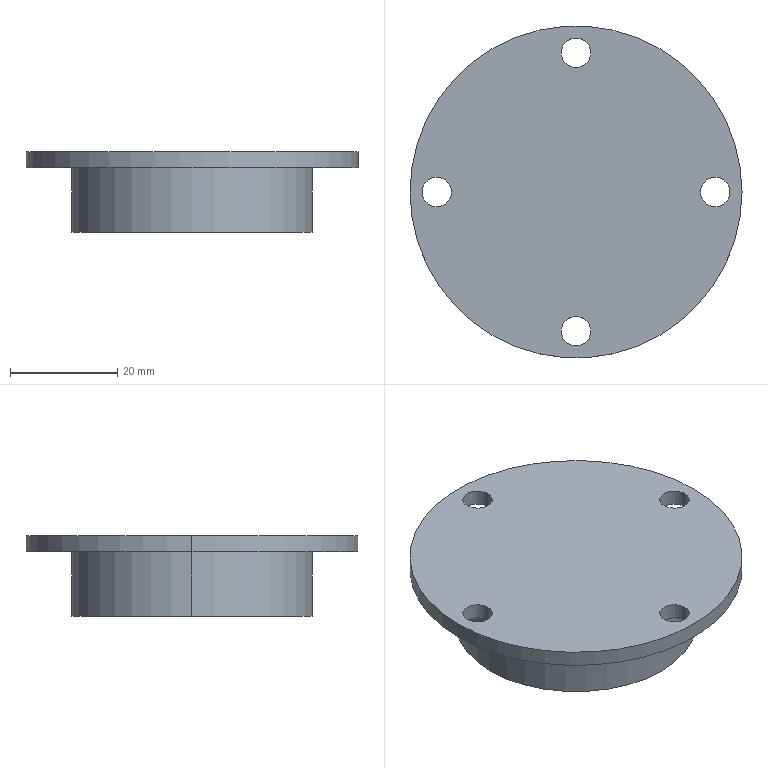Part | SolidWorks | features ICE 2, Cut 1, Extrusion 1 | 1 solid | 18 faces | box 62 x 62 x 15 mm | volume 19198 mm3 | cylinder 14 | plane 4 | commonest cylinder face diameters 5.5 x8 35 x2 45 x2 62 x2
STEP:
#1=CARTESIAN_POINT('',(-52.75,26.,-694.19));
#2=VERTEX_POINT('',#1);
#3=CARTESIAN_POINT('',(-47.25,26.,-694.19));
#4=VERTEX_POINT('',#3);
#5=CARTESIAN_POINT('',(-50.,26.,-694.19));
#6=DIRECTION('',(0.,0.,1.));
#7=DIRECTION('',(1.,0.,0.));
#8=AXIS2_PLACEMENT_3D('',#5,#6,#7);
#9=CIRCLE('',#8,2.75);
#10=EDGE_CURVE('',#2,#4,#9,.T.);
#11=ORIENTED_EDGE('',*,*,#10,.F.);
#12=CARTESIAN_POINT('',(-52.75,26.,-691.19));
#13=VERTEX_POINT('',#12);
#14=CARTESIAN_POINT('',(-52.75,26.,-703.19));
#15=DIRECTION('',(0.,0.,1.));
#16=VECTOR('',#15,1000.);
#17=LINE('',#14,#16);
#18=EDGE_CURVE('',#2,#13,#17,.T.);
#19=ORIENTED_EDGE('',*,*,#18,.T.);
#20=CARTESIAN_POINT('',(-47.25,26.,-691.19));
#21=VERTEX_POINT('',#20);
#22=CARTESIAN_POINT('',(-50.,26.,-691.19));
#23=DIRECTION('',(0.,0.,1.));
#24=DIRECTION('',(1.,0.,0.));
#25=AXIS2_PLACEMENT_3D('',#22,#23,#24);
#26=CIRCLE('',#25,2.75);
#27=EDGE_CURVE('',#13,#21,#26,.T.);
#28=ORIENTED_EDGE('',*,*,#27,.T.);
#29=CARTESIAN_POINT('',(-47.25,26.,-703.19));
#30=DIRECTION('',(0.,0.,1.));
#31=VECTOR('',#30,1000.);
#32=LINE('',#29,#31);
#33=EDGE_CURVE('',#4,#21,#32,.T.);
#34=ORIENTED_EDGE('',*,*,#33,.F.);
#35=EDGE_LOOP('',(#11,#19,#28,#34));
#36=FACE_OUTER_BOUND('',#35,.T.);
#37=CARTESIAN_POINT('',(-50.,26.,-703.19));
#38=DIRECTION('',(0.,0.,1.));
#39=DIRECTION('',(1.,0.,0.));
#40=AXIS2_PLACEMENT_3D('',#37,#38,#39);
#41=CYLINDRICAL_SURFACE('',#40,2.75);
#42=ADVANCED_FACE('',(#36),#41,.F.);
#43=CARTESIAN_POINT('',(-26.75,0.,-694.19));
#44=VERTEX_POINT('',#43);
#45=CARTESIAN_POINT('',(-21.25,0.,-694.19));
#46=VERTEX_POINT('',#45);
#47=CARTESIAN_POINT('',(-24.,0.,-694.19));
#48=DIRECTION('',(0.,0.,1.));
#49=DIRECTION('',(1.,0.,0.));
#50=AXIS2_PLACEMENT_3D('',#47,#48,#49);
#51=CIRCLE('',#50,2.75);
#52=EDGE_CURVE('',#44,#46,#51,.T.);
#53=ORIENTED_EDGE('',*,*,#52,.F.);
#54=CARTESIAN_POINT('',(-26.75,0.,-691.19));
#55=VERTEX_POINT('',#54);
#56=CARTESIAN_POINT('',(-26.75,0.,-703.19));
#57=DIRECTION('',(0.,0.,1.));
#58=VECTOR('',#57,1000.);
#59=LINE('',#56,#58);
#60=EDGE_CURVE('',#44,#55,#59,.T.);
#61=ORIENTED_EDGE('',*,*,#60,.T.);
#62=CARTESIAN_POINT('',(-21.25,0.,-691.19));
#63=VERTEX_POINT('',#62);
#64=CARTESIAN_POINT('',(-24.,0.,-691.19));
#65=DIRECTION('',(0.,0.,1.));
#66=DIRECTION('',(1.,0.,0.));
#67=AXIS2_PLACEMENT_3D('',#64,#65,#66);
#68=CIRCLE('',#67,2.75);
#69=EDGE_CURVE('',#55,#63,#68,.T.);
#70=ORIENTED_EDGE('',*,*,#69,.T.);
#71=CARTESIAN_POINT('',(-21.25,0.,-703.19));
#72=DIRECTION('',(0.,0.,1.));
#73=VECTOR('',#72,1000.);
#74=LINE('',#71,#73);
#75=EDGE_CURVE('',#46,#63,#74,.T.);
#76=ORIENTED_EDGE('',*,*,#75,.F.);
#77=EDGE_LOOP('',(#53,#61,#70,#76));
#78=FACE_OUTER_BOUND('',#77,.T.);
#79=CARTESIAN_POINT('',(-24.,0.,-703.19));
#80=DIRECTION('',(0.,0.,1.));
#81=DIRECTION('',(1.,0.,0.));
#82=AXIS2_PLACEMENT_3D('',#79,#80,#81);
#83=CYLINDRICAL_SURFACE('',#82,2.75);
#84=ADVANCED_FACE('',(#78),#83,.F.);
#85=CARTESIAN_POINT('',(-52.75,-26.,-694.19));
#86=VERTEX_POINT('',#85);
#87=CARTESIAN_POINT('',(-47.25,-26.,-694.19));
#88=VERTEX_POINT('',#87);
#89=CARTESIAN_POINT('',(-50.,-26.,-694.19));
#90=DIRECTION('',(0.,0.,1.));
#91=DIRECTION('',(1.,0.,0.));
#92=AXIS2_PLACEMENT_3D('',#89,#90,#91);
#93=CIRCLE('',#92,2.75);
#94=EDGE_CURVE('',#86,#88,#93,.T.);
#95=ORIENTED_EDGE('',*,*,#94,.F.);
#96=CARTESIAN_POINT('',(-52.75,-26.,-691.19));
#97=VERTEX_POINT('',#96);
#98=CARTESIAN_POINT('',(-52.75,-26.,-703.19));
#99=DIRECTION('',(0.,0.,1.));
#100=VECTOR('',#99,1000.);
#101=LINE('',#98,#100);
#102=EDGE_CURVE('',#86,#97,#101,.T.);
#103=ORIENTED_EDGE('',*,*,#102,.T.);
#104=CARTESIAN_POINT('',(-47.25,-26.,-691.19));
#105=VERTEX_POINT('',#104);
#106=CARTESIAN_POINT('',(-50.,-26.,-691.19));
#107=DIRECTION('',(0.,0.,1.));
#108=DIRECTION('',(1.,0.,0.));
#109=AXIS2_PLACEMENT_3D('',#106,#107,#108);
#110=CIRCLE('',#109,2.75);
#111=EDGE_CURVE('',#97,#105,#110,.T.);
#112=ORIENTED_EDGE('',*,*,#111,.T.);
#113=CARTESIAN_POINT('',(-47.25,-26.,-703.19));
#114=DIRECTION('',(0.,0.,1.));
#115=VECTOR('',#114,1000.);
#116=LINE('',#113,#115);
#117=EDGE_CURVE('',#88,#105,#116,.T.);
#118=ORIENTED_EDGE('',*,*,#117,.F.);
#119=EDGE_LOOP('',(#95,#103,#112,#118));
#120=FACE_OUTER_BOUND('',#119,.T.);
#121=CARTESIAN_POINT('',(-50.,-26.,-703.19));
#122=DIRECTION('',(0.,0.,1.));
#123=DIRECTION('',(1.,0.,0.));
#124=AXIS2_PLACEMENT_3D('',#121,#122,#123);
#125=CYLINDRICAL_SURFACE('',#124,2.75);
#126=ADVANCED_FACE('',(#120),#125,.F.);
#127=CARTESIAN_POINT('',(-78.75,0.,-694.19));
#128=VERTEX_POINT('',#127);
#129=CARTESIAN_POINT('',(-73.25,0.,-694.19));
#130=VERTEX_POINT('',#129);
#131=CARTESIAN_POINT('',(-76.,0.,-694.19));
#132=DIRECTION('',(0.,0.,1.));
#133=DIRECTION('',(1.,0.,0.));
#134=AXIS2_PLACEMENT_3D('',#131,#132,#133);
#135=CIRCLE('',#134,2.75);
#136=EDGE_CURVE('',#128,#130,#135,.T.);
#137=ORIENTED_EDGE('',*,*,#136,.F.);
#138=CARTESIAN_POINT('',(-78.75,0.,-691.19));
#139=VERTEX_POINT('',#138);
#140=CARTESIAN_POINT('',(-78.75,0.,-703.19));
#141=DIRECTION('',(0.,0.,1.));
#142=VECTOR('',#141,1000.);
#143=LINE('',#140,#142);
#144=EDGE_CURVE('',#128,#139,#143,.T.);
#145=ORIENTED_EDGE('',*,*,#144,.T.);
#146=CARTESIAN_POINT('',(-73.25,0.,-691.19));
#147=VERTEX_POINT('',#146);
#148=CARTESIAN_POINT('',(-76.,0.,-691.19));
#149=DIRECTION('',(0.,0.,1.));
#150=DIRECTION('',(1.,0.,0.));
#151=AXIS2_PLACEMENT_3D('',#148,#149,#150);
#152=CIRCLE('',#151,2.75);
#153=EDGE_CURVE('',#139,#147,#152,.T.);
#154=ORIENTED_EDGE('',*,*,#153,.T.);
#155=CARTESIAN_POINT('',(-73.25,0.,-703.19));
#156=DIRECTION('',(0.,0.,1.));
#157=VECTOR('',#156,1000.);
#158=LINE('',#155,#157);
#159=EDGE_CURVE('',#130,#147,#158,.T.);
#160=ORIENTED_EDGE('',*,*,#159,.F.);
#161=EDGE_LOOP('',(#137,#145,#154,#160));
#162=FACE_OUTER_BOUND('',#161,.T.);
#163=CARTESIAN_POINT('',(-76.,0.,-703.19));
#164=DIRECTION('',(0.,0.,1.));
#165=DIRECTION('',(1.,0.,0.));
#166=AXIS2_PLACEMENT_3D('',#163,#164,#165);
#167=CYLINDRICAL_SURFACE('',#166,2.75);
#168=ADVANCED_FACE('',(#162),#167,.F.);
#169=CARTESIAN_POINT('',(-32.5,0.,-697.19));
#170=VERTEX_POINT('',#169);
#171=CARTESIAN_POINT('',(-67.5,0.,-697.19));
#172=VERTEX_POINT('',#171);
#173=CARTESIAN_POINT('',(-50.,0.,-697.19));
#174=DIRECTION('',(0.,0.,-1.));
#175=DIRECTION('',(-1.,0.,0.));
#176=AXIS2_PLACEMENT_3D('',#173,#174,#175);
#177=CIRCLE('',#176,17.5);
#178=EDGE_CURVE('',#170,#172,#177,.T.);
#179=ORIENTED_EDGE('',*,*,#178,.F.);
#180=CARTESIAN_POINT('',(-32.5,0.,-706.19));
#181=VERTEX_POINT('',#180);
#182=CARTESIAN_POINT('',(-32.5,0.,-697.19));
#183=DIRECTION('',(0.,0.,-1.));
#184=VECTOR('',#183,1000.);
#185=LINE('',#182,#184);
#186=EDGE_CURVE('',#170,#181,#185,.T.);
#187=ORIENTED_EDGE('',*,*,#186,.T.);
#188=CARTESIAN_POINT('',(-67.5,0.,-706.19));
#189=VERTEX_POINT('',#188);
#190=CARTESIAN_POINT('',(-50.,0.,-706.19));
#191=DIRECTION('',(0.,0.,-1.));
#192=DIRECTION('',(-1.,0.,0.));
#193=AXIS2_PLACEMENT_3D('',#190,#191,#192);
#194=CIRCLE('',#193,17.5);
#195=EDGE_CURVE('',#181,#189,#194,.T.);
#196=ORIENTED_EDGE('',*,*,#195,.T.);
#197=CARTESIAN_POINT('',(-67.5,0.,-697.19));
#198=DIRECTION('',(0.,0.,-1.));
#199=VECTOR('',#198,1000.);
#200=LINE('',#197,#199);
#201=EDGE_CURVE('',#172,#189,#200,.T.);
#202=ORIENTED_EDGE('',*,*,#201,.F.);
#203=EDGE_LOOP('',(#179,#187,#196,#202));
#204=FACE_OUTER_BOUND('',#203,.T.);
#205=CARTESIAN_POINT('',(-50.,0.,-697.19));
#206=DIRECTION('',(0.,0.,-1.));
#207=DIRECTION('',(-1.,0.,0.));
#208=AXIS2_PLACEMENT_3D('',#205,#206,#207);
#209=CYLINDRICAL_SURFACE('',#208,17.5);
#210=ADVANCED_FACE('',(#204),#209,.F.);
#211=CARTESIAN_POINT('',(-72.5,0.,-706.19));
#212=VERTEX_POINT('',#211);
#213=CARTESIAN_POINT('',(-27.5,0.,-706.19));
#214=VERTEX_POINT('',#213);
#215=CARTESIAN_POINT('',(-50.,0.,-706.19));
#216=DIRECTION('',(0.,0.,-1.));
#217=DIRECTION('',(-1.,0.,0.));
#218=AXIS2_PLACEMENT_3D('',#215,#216,#217);
#219=CIRCLE('',#218,22.5);
#220=EDGE_CURVE('',#212,#214,#219,.T.);
#221=ORIENTED_EDGE('',*,*,#220,.F.);
#222=CARTESIAN_POINT('',(-72.5,0.,-694.19));
#223=VERTEX_POINT('',#222);
#224=CARTESIAN_POINT('',(-72.5,0.,-706.19));
#225=DIRECTION('',(0.,0.,1.));
#226=VECTOR('',#225,1000.);
#227=LINE('',#224,#226);
#228=EDGE_CURVE('',#212,#223,#227,.T.);
#229=ORIENTED_EDGE('',*,*,#228,.T.);
#230=CARTESIAN_POINT('',(-27.5,0.,-694.19));
#231=VERTEX_POINT('',#230);
#232=CARTESIAN_POINT('',(-50.,0.,-694.19));
#233=DIRECTION('',(0.,0.,-1.));
#234=DIRECTION('',(-1.,0.,0.));
#235=AXIS2_PLACEMENT_3D('',#232,#233,#234);
#236=CIRCLE('',#235,22.5);
#237=EDGE_CURVE('',#223,#231,#236,.T.);
#238=ORIENTED_EDGE('',*,*,#237,.T.);
#239=CARTESIAN_POINT('',(-27.5,0.,-706.19));
#240=DIRECTION('',(0.,0.,1.));
#241=VECTOR('',#240,1000.);
#242=LINE('',#239,#241);
#243=EDGE_CURVE('',#214,#231,#242,.T.);
#244=ORIENTED_EDGE('',*,*,#243,.F.);
#245=EDGE_LOOP('',(#221,#229,#238,#244));
#246=FACE_OUTER_BOUND('',#245,.T.);
#247=CARTESIAN_POINT('',(-50.,0.,-706.19));
#248=DIRECTION('',(0.,0.,1.));
#249=DIRECTION('',(1.,0.,0.));
#250=AXIS2_PLACEMENT_3D('',#247,#248,#249);
#251=CYLINDRICAL_SURFACE('',#250,22.5);
#252=ADVANCED_FACE('',(#246),#251,.T.);
#253=CARTESIAN_POINT('',(-19.,0.,-691.19));
#254=VERTEX_POINT('',#253);
#255=CARTESIAN_POINT('',(-81.,0.,-691.19));
#256=VERTEX_POINT('',#255);
#257=CARTESIAN_POINT('',(-50.,0.,-691.19));
#258=DIRECTION('',(0.,0.,1.));
#259=DIRECTION('',(1.,0.,0.));
#260=AXIS2_PLACEMENT_3D('',#257,#258,#259);
#261=CIRCLE('',#260,31.);
#262=EDGE_CURVE('',#254,#256,#261,.T.);
#263=ORIENTED_EDGE('',*,*,#262,.F.);
#264=CARTESIAN_POINT('',(-19.,0.,-694.19));
#265=VERTEX_POINT('',#264);
#266=CARTESIAN_POINT('',(-19.,0.,-691.19));
#267=DIRECTION('',(0.,0.,-1.));
#268=VECTOR('',#267,1000.);
#269=LINE('',#266,#268);
#270=EDGE_CURVE('',#254,#265,#269,.T.);
#271=ORIENTED_EDGE('',*,*,#270,.T.);
#272=CARTESIAN_POINT('',(-81.,0.,-694.19));
#273=VERTEX_POINT('',#272);
#274=CARTESIAN_POINT('',(-50.,0.,-694.19));
#275=DIRECTION('',(0.,0.,1.));
#276=DIRECTION('',(1.,0.,0.));
#277=AXIS2_PLACEMENT_3D('',#274,#275,#276);
#278=CIRCLE('',#277,31.);
#279=EDGE_CURVE('',#265,#273,#278,.T.);
#280=ORIENTED_EDGE('',*,*,#279,.T.);
#281=CARTESIAN_POINT('',(-81.,0.,-691.19));
#282=DIRECTION('',(0.,0.,-1.));
#283=VECTOR('',#282,1000.);
#284=LINE('',#281,#283);
#285=EDGE_CURVE('',#256,#273,#284,.T.);
#286=ORIENTED_EDGE('',*,*,#285,.F.);
#287=EDGE_LOOP('',(#263,#271,#280,#286));
#288=FACE_OUTER_BOUND('',#287,.T.);
#289=CARTESIAN_POINT('',(-50.,0.,-691.19));
#290=DIRECTION('',(0.,0.,-1.));
#291=DIRECTION('',(-1.,0.,0.));
#292=AXIS2_PLACEMENT_3D('',#289,#290,#291);
#293=CYLINDRICAL_SURFACE('',#292,31.);
#294=ADVANCED_FACE('',(#288),#293,.T.);
#295=ORIENTED_EDGE('',*,*,#270,.F.);
#296=CARTESIAN_POINT('',(-50.,0.,-691.19));
#297=DIRECTION('',(0.,0.,1.));
#298=DIRECTION('',(1.,0.,0.));
#299=AXIS2_PLACEMENT_3D('',#296,#297,#298);
#300=CIRCLE('',#299,31.);
#301=EDGE_CURVE('',#256,#254,#300,.T.);
#302=ORIENTED_EDGE('',*,*,#301,.F.);
#303=ORIENTED_EDGE('',*,*,#285,.T.);
#304=CARTESIAN_POINT('',(-50.,0.,-694.19));
#305=DIRECTION('',(0.,0.,1.));
#306=DIRECTION('',(1.,0.,0.));
#307=AXIS2_PLACEMENT_3D('',#304,#305,#306);
#308=CIRCLE('',#307,31.);
#309=EDGE_CURVE('',#273,#265,#308,.T.);
#310=ORIENTED_EDGE('',*,*,#309,.T.);
#311=EDGE_LOOP('',(#295,#302,#303,#310));
#312=FACE_OUTER_BOUND('',#311,.T.);
#313=CARTESIAN_POINT('',(-50.,0.,-691.19));
#314=DIRECTION('',(0.,0.,-1.));
#315=DIRECTION('',(-1.,0.,0.));
#316=AXIS2_PLACEMENT_3D('',#313,#314,#315);
#317=CYLINDRICAL_SURFACE('',#316,31.);
#318=ADVANCED_FACE('',(#312),#317,.T.);
#319=CARTESIAN_POINT('',(-50.,26.,-691.19));
#320=DIRECTION('',(0.,0.,1.));
#321=DIRECTION('',(1.,0.,0.));
#322=AXIS2_PLACEMENT_3D('',#319,#320,#321);
#323=CIRCLE('',#322,2.75);
#324=EDGE_CURVE('',#21,#13,#323,.T.);
#325=ORIENTED_EDGE('',*,*,#324,.F.);
#326=ORIENTED_EDGE('',*,*,#27,.F.);
#327=EDGE_LOOP('',(#325,#326));
#328=FACE_BOUND('',#327,.T.);
#329=CARTESIAN_POINT('',(-24.,0.,-691.19));
#330=DIRECTION('',(0.,0.,1.));
#331=DIRECTION('',(1.,0.,0.));
#332=AXIS2_PLACEMENT_3D('',#329,#330,#331);
#333=CIRCLE('',#332,2.75);
#334=EDGE_CURVE('',#63,#55,#333,.T.);
#335=ORIENTED_EDGE('',*,*,#334,.F.);
#336=ORIENTED_EDGE('',*,*,#69,.F.);
#337=EDGE_LOOP('',(#335,#336));
#338=FACE_BOUND('',#337,.T.);
#339=CARTESIAN_POINT('',(-50.,-26.,-691.19));
#340=DIRECTION('',(0.,0.,1.));
#341=DIRECTION('',(1.,0.,0.));
#342=AXIS2_PLACEMENT_3D('',#339,#340,#341);
#343=CIRCLE('',#342,2.75);
#344=EDGE_CURVE('',#105,#97,#343,.T.);
#345=ORIENTED_EDGE('',*,*,#344,.F.);
#346=ORIENTED_EDGE('',*,*,#111,.F.);
#347=EDGE_LOOP('',(#345,#346));
#348=FACE_BOUND('',#347,.T.);
#349=CARTESIAN_POINT('',(-76.,0.,-691.19));
#350=DIRECTION('',(0.,0.,1.));
#351=DIRECTION('',(1.,0.,0.));
#352=AXIS2_PLACEMENT_3D('',#349,#350,#351);
#353=CIRCLE('',#352,2.75);
#354=EDGE_CURVE('',#147,#139,#353,.T.);
#355=ORIENTED_EDGE('',*,*,#354,.F.);
#356=ORIENTED_EDGE('',*,*,#153,.F.);
#357=EDGE_LOOP('',(#355,#356));
#358=FACE_BOUND('',#357,.T.);
#359=ORIENTED_EDGE('',*,*,#301,.T.);
#360=ORIENTED_EDGE('',*,*,#262,.T.);
#361=EDGE_LOOP('',(#359,#360));
#362=FACE_OUTER_BOUND('',#361,.T.);
#363=CARTESIAN_POINT('',(-50.,0.,-691.19));
#364=DIRECTION('',(0.,0.,1.));
#365=DIRECTION('',(1.,0.,0.));
#366=AXIS2_PLACEMENT_3D('',#363,#364,#365);
#367=PLANE('',#366);
#368=ADVANCED_FACE('',(#328,#338,#348,#358,#362),#367,.T.);
#369=CARTESIAN_POINT('',(-50.,26.,-694.19));
#370=DIRECTION('',(0.,0.,1.));
#371=DIRECTION('',(1.,0.,0.));
#372=AXIS2_PLACEMENT_3D('',#369,#370,#371);
#373=CIRCLE('',#372,2.75);
#374=EDGE_CURVE('',#4,#2,#373,.T.);
#375=ORIENTED_EDGE('',*,*,#374,.T.);
#376=ORIENTED_EDGE('',*,*,#10,.T.);
#377=EDGE_LOOP('',(#375,#376));
#378=FACE_BOUND('',#377,.T.);
#379=CARTESIAN_POINT('',(-24.,0.,-694.19));
#380=DIRECTION('',(0.,0.,1.));
#381=DIRECTION('',(1.,0.,0.));
#382=AXIS2_PLACEMENT_3D('',#379,#380,#381);
#383=CIRCLE('',#382,2.75);
#384=EDGE_CURVE('',#46,#44,#383,.T.);
#385=ORIENTED_EDGE('',*,*,#384,.T.);
#386=ORIENTED_EDGE('',*,*,#52,.T.);
#387=EDGE_LOOP('',(#385,#386));
#388=FACE_BOUND('',#387,.T.);
#389=CARTESIAN_POINT('',(-50.,-26.,-694.19));
#390=DIRECTION('',(0.,0.,1.));
#391=DIRECTION('',(1.,0.,0.));
#392=AXIS2_PLACEMENT_3D('',#389,#390,#391);
#393=CIRCLE('',#392,2.75);
#394=EDGE_CURVE('',#88,#86,#393,.T.);
#395=ORIENTED_EDGE('',*,*,#394,.T.);
#396=ORIENTED_EDGE('',*,*,#94,.T.);
#397=EDGE_LOOP('',(#395,#396));
#398=FACE_BOUND('',#397,.T.);
#399=CARTESIAN_POINT('',(-76.,0.,-694.19));
#400=DIRECTION('',(0.,0.,1.));
#401=DIRECTION('',(1.,0.,0.));
#402=AXIS2_PLACEMENT_3D('',#399,#400,#401);
#403=CIRCLE('',#402,2.75);
#404=EDGE_CURVE('',#130,#128,#403,.T.);
#405=ORIENTED_EDGE('',*,*,#404,.T.);
#406=ORIENTED_EDGE('',*,*,#136,.T.);
#407=EDGE_LOOP('',(#405,#406));
#408=FACE_BOUND('',#407,.T.);
#409=CARTESIAN_POINT('',(-50.,0.,-694.19));
#410=DIRECTION('',(0.,0.,-1.));
#411=DIRECTION('',(-1.,0.,0.));
#412=AXIS2_PLACEMENT_3D('',#409,#410,#411);
#413=CIRCLE('',#412,22.5);
#414=EDGE_CURVE('',#231,#223,#413,.T.);
#415=ORIENTED_EDGE('',*,*,#414,.F.);
#416=ORIENTED_EDGE('',*,*,#237,.F.);
#417=EDGE_LOOP('',(#415,#416));
#418=FACE_BOUND('',#417,.T.);
#419=ORIENTED_EDGE('',*,*,#309,.F.);
#420=ORIENTED_EDGE('',*,*,#279,.F.);
#421=EDGE_LOOP('',(#419,#420));
#422=FACE_OUTER_BOUND('',#421,.T.);
#423=CARTESIAN_POINT('',(-50.,0.,-694.19));
#424=DIRECTION('',(0.,0.,1.));
#425=DIRECTION('',(1.,0.,0.));
#426=AXIS2_PLACEMENT_3D('',#423,#424,#425);
#427=PLANE('',#426);
#428=ADVANCED_FACE('',(#378,#388,#398,#408,#418,#422),#427,.F.);
#429=ORIENTED_EDGE('',*,*,#228,.F.);
#430=CARTESIAN_POINT('',(-50.,0.,-706.19));
#431=DIRECTION('',(0.,0.,-1.));
#432=DIRECTION('',(-1.,0.,0.));
#433=AXIS2_PLACEMENT_3D('',#430,#431,#432);
#434=CIRCLE('',#433,22.5);
#435=EDGE_CURVE('',#214,#212,#434,.T.);
#436=ORIENTED_EDGE('',*,*,#435,.F.);
#437=ORIENTED_EDGE('',*,*,#243,.T.);
#438=ORIENTED_EDGE('',*,*,#414,.T.);
#439=EDGE_LOOP('',(#429,#436,#437,#438));
#440=FACE_OUTER_BOUND('',#439,.T.);
#441=CARTESIAN_POINT('',(-50.,0.,-706.19));
#442=DIRECTION('',(0.,0.,1.));
#443=DIRECTION('',(1.,0.,0.));
#444=AXIS2_PLACEMENT_3D('',#441,#442,#443);
#445=CYLINDRICAL_SURFACE('',#444,22.5);
#446=ADVANCED_FACE('',(#440),#445,.T.);
#447=CARTESIAN_POINT('',(-50.,0.,-706.19));
#448=DIRECTION('',(0.,0.,-1.));
#449=DIRECTION('',(-1.,0.,0.));
#450=AXIS2_PLACEMENT_3D('',#447,#448,#449);
#451=CIRCLE('',#450,17.5);
#452=EDGE_CURVE('',#189,#181,#451,.T.);
#453=ORIENTED_EDGE('',*,*,#452,.F.);
#454=ORIENTED_EDGE('',*,*,#195,.F.);
#455=EDGE_LOOP('',(#453,#454));
#456=FACE_BOUND('',#455,.T.);
#457=ORIENTED_EDGE('',*,*,#435,.T.);
#458=ORIENTED_EDGE('',*,*,#220,.T.);
#459=EDGE_LOOP('',(#457,#458));
#460=FACE_OUTER_BOUND('',#459,.T.);
#461=CARTESIAN_POINT('',(-50.,0.,-706.19));
#462=DIRECTION('',(0.,0.,-1.));
#463=DIRECTION('',(-1.,0.,0.));
#464=AXIS2_PLACEMENT_3D('',#461,#462,#463);
#465=PLANE('',#464);
#466=ADVANCED_FACE('',(#456,#460),#465,.T.);
#467=ORIENTED_EDGE('',*,*,#186,.F.);
#468=CARTESIAN_POINT('',(-50.,0.,-697.19));
#469=DIRECTION('',(0.,0.,-1.));
#470=DIRECTION('',(-1.,0.,0.));
#471=AXIS2_PLACEMENT_3D('',#468,#469,#470);
#472=CIRCLE('',#471,17.5);
#473=EDGE_CURVE('',#172,#170,#472,.T.);
#474=ORIENTED_EDGE('',*,*,#473,.F.);
#475=ORIENTED_EDGE('',*,*,#201,.T.);
#476=ORIENTED_EDGE('',*,*,#452,.T.);
#477=EDGE_LOOP('',(#467,#474,#475,#476));
#478=FACE_OUTER_BOUND('',#477,.T.);
#479=CARTESIAN_POINT('',(-50.,0.,-697.19));
#480=DIRECTION('',(0.,0.,-1.));
#481=DIRECTION('',(-1.,0.,0.));
#482=AXIS2_PLACEMENT_3D('',#479,#480,#481);
#483=CYLINDRICAL_SURFACE('',#482,17.5);
#484=ADVANCED_FACE('',(#478),#483,.F.);
#485=ORIENTED_EDGE('',*,*,#473,.T.);
#486=ORIENTED_EDGE('',*,*,#178,.T.);
#487=EDGE_LOOP('',(#485,#486));
#488=FACE_OUTER_BOUND('',#487,.T.);
#489=CARTESIAN_POINT('',(-50.,0.,-697.19));
#490=DIRECTION('',(0.,0.,-1.));
#491=DIRECTION('',(-1.,0.,0.));
#492=AXIS2_PLACEMENT_3D('',#489,#490,#491);
#493=PLANE('',#492);
#494=ADVANCED_FACE('',(#488),#493,.T.);
#495=ORIENTED_EDGE('',*,*,#144,.F.);
#496=ORIENTED_EDGE('',*,*,#404,.F.);
#497=ORIENTED_EDGE('',*,*,#159,.T.);
#498=ORIENTED_EDGE('',*,*,#354,.T.);
#499=EDGE_LOOP('',(#495,#496,#497,#498));
#500=FACE_OUTER_BOUND('',#499,.T.);
#501=CARTESIAN_POINT('',(-76.,0.,-703.19));
#502=DIRECTION('',(0.,0.,1.));
#503=DIRECTION('',(1.,0.,0.));
#504=AXIS2_PLACEMENT_3D('',#501,#502,#503);
#505=CYLINDRICAL_SURFACE('',#504,2.75);
#506=ADVANCED_FACE('',(#500),#505,.F.);
#507=ORIENTED_EDGE('',*,*,#102,.F.);
#508=ORIENTED_EDGE('',*,*,#394,.F.);
#509=ORIENTED_EDGE('',*,*,#117,.T.);
#510=ORIENTED_EDGE('',*,*,#344,.T.);
#511=EDGE_LOOP('',(#507,#508,#509,#510));
#512=FACE_OUTER_BOUND('',#511,.T.);
#513=CARTESIAN_POINT('',(-50.,-26.,-703.19));
#514=DIRECTION('',(0.,0.,1.));
#515=DIRECTION('',(1.,0.,0.));
#516=AXIS2_PLACEMENT_3D('',#513,#514,#515);
#517=CYLINDRICAL_SURFACE('',#516,2.75);
#518=ADVANCED_FACE('',(#512),#517,.F.);
#519=ORIENTED_EDGE('',*,*,#60,.F.);
#520=ORIENTED_EDGE('',*,*,#384,.F.);
#521=ORIENTED_EDGE('',*,*,#75,.T.);
#522=ORIENTED_EDGE('',*,*,#334,.T.);
#523=EDGE_LOOP('',(#519,#520,#521,#522));
#524=FACE_OUTER_BOUND('',#523,.T.);
#525=CARTESIAN_POINT('',(-24.,0.,-703.19));
#526=DIRECTION('',(0.,0.,1.));
#527=DIRECTION('',(1.,0.,0.));
#528=AXIS2_PLACEMENT_3D('',#525,#526,#527);
#529=CYLINDRICAL_SURFACE('',#528,2.75);
#530=ADVANCED_FACE('',(#524),#529,.F.);
#531=ORIENTED_EDGE('',*,*,#18,.F.);
#532=ORIENTED_EDGE('',*,*,#374,.F.);
#533=ORIENTED_EDGE('',*,*,#33,.T.);
#534=ORIENTED_EDGE('',*,*,#324,.T.);
#535=EDGE_LOOP('',(#531,#532,#533,#534));
#536=FACE_OUTER_BOUND('',#535,.T.);
#537=CARTESIAN_POINT('',(-50.,26.,-703.19));
#538=DIRECTION('',(0.,0.,1.));
#539=DIRECTION('',(1.,0.,0.));
#540=AXIS2_PLACEMENT_3D('',#537,#538,#539);
#541=CYLINDRICAL_SURFACE('',#540,2.75);
#542=ADVANCED_FACE('',(#536),#541,.F.);
#543=CLOSED_SHELL('',(#42,#84,#126,#168,#210,#252,#294,#318,#368,#428,#446,#466,#484,#494,#506,#518,#530,#542));
#544=MANIFOLD_SOLID_BREP('',#543);
#545=CARTESIAN_POINT('',(0.,0.,0.));
#546=DIRECTION('',(0.,0.,1.));
#547=DIRECTION('',(1.,0.,0.));
#548=AXIS2_PLACEMENT_3D('',#545,#546,#547);
#549=(LENGTH_UNIT()NAMED_UNIT(*)SI_UNIT(.MILLI.,.METRE.));
#550=UNCERTAINTY_MEASURE_WITH_UNIT(LENGTH_MEASURE(0.00001),#549,'','');
#551=(NAMED_UNIT(*)PLANE_ANGLE_UNIT()SI_UNIT($,.RADIAN.));
#552=(NAMED_UNIT(*)SI_UNIT($,.STERADIAN.)SOLID_ANGLE_UNIT());
#553=(GEOMETRIC_REPRESENTATION_CONTEXT(3)GLOBAL_UNCERTAINTY_ASSIGNED_CONTEXT((#550))GLOBAL_UNIT_ASSIGNED_CONTEXT((#549,#551,#552))REPRESENTATION_CONTEXT('',''));
#554=ADVANCED_BREP_SHAPE_REPRESENTATION('',(#544,#548),#553);